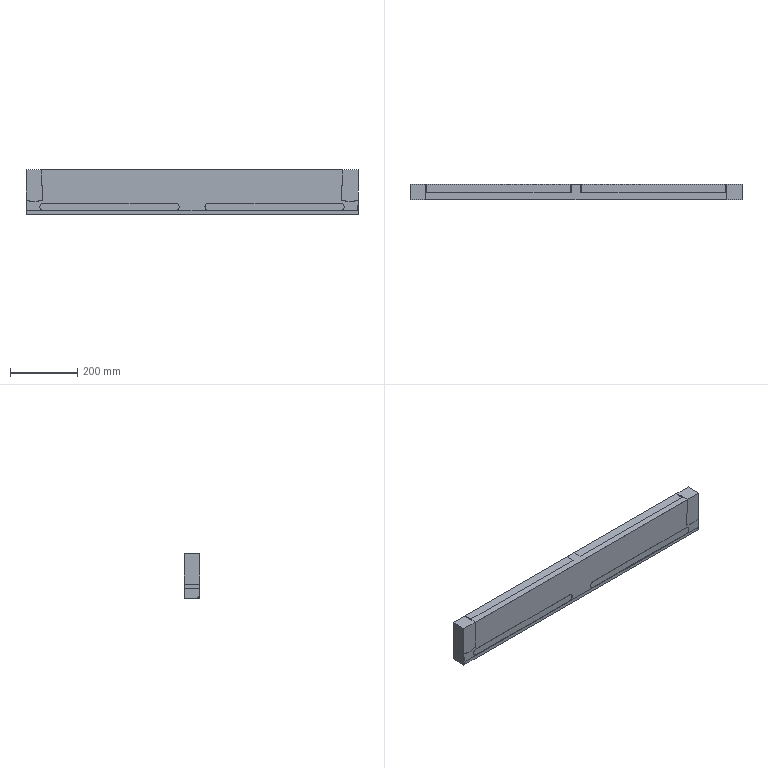NC program | NX | posted with a generic post | part box 987 x 45 x 132.5 mm
Whole program:
N10 G17 G21 G94 G90
(ZLEVEL_PROFILE_2 , TOOL : D12)
N12 T20 M6
N14 G54
N16 G17 G0 G90 X-178.716 Y48.65 B0. C0. S7500 M3
N18 G43 Z30. H20
N20 Z1.5
N22 G94 G1 X-245.5 Z-2. F1001.
N24 X-441. F3000.
N26 G3 X-445.4 Y44.25 R4.4
N28 X-441. Y39.85 R4.4
N30 G1 X-50.
N32 G3 X-45.6 Y44.25 R4.4
N34 X-50. Y48.65 R4.4
N36 G1 X-245.5
N38 X-360.08 Z-4.
N40 X-441.
N42 G3 X-445.4 Y44.25 R4.4
N44 X-441. Y39.85 R4.4
N46 G1 X-50.
N48 G3 X-45.6 Y44.25 R4.4
N50 X-50. Y48.65 R4.4
N52 G1 X-245.5
N54 X-360.08 Z-6.
N56 X-441.
N58 G3 X-445.4 Y44.25 R4.4
N60 X-441. Y39.85 R4.4
N62 G1 X-50.
N64 G3 X-45.6 Y44.25 R4.4
N66 X-50. Y48.65 R4.4
N68 G1 X-245.5
N70 X-360.08 Z-8.
N72 X-441.
N74 G3 X-445.4 Y44.25 R4.4
N76 X-441. Y39.85 R4.4
N78 G1 X-50.
N80 G3 X-45.6 Y44.25 R4.4
N82 X-50. Y48.65 R4.4
N84 G1 X-245.5
N86 X-360.08 Z-10.
N88 X-441.
N90 G3 X-445.4 Y44.25 R4.4
N92 X-441. Y39.85 R4.4
N94 G1 X-50.
N96 G3 X-45.6 Y44.25 R4.4
N98 X-50. Y48.65 R4.4
N100 G1 X-245.5
N102 X-360.08 Z-12.
N104 X-441.
N106 G3 X-445.4 Y44.25 R4.4
N108 X-441. Y39.85 R4.4
N110 G1 X-50.
N112 G3 X-45.6 Y44.25 R4.4
N114 X-50. Y48.65 R4.4
N116 G1 X-245.5
N118 X-360.08 Z-14.
N120 X-441.
N122 G3 X-445.4 Y44.25 R4.4
N124 X-441. Y39.85 R4.4
N126 G1 X-50.
N128 G3 X-45.6 Y44.25 R4.4
N130 X-50. Y48.65 R4.4
N132 G1 X-245.5
N134 X-360.08 Z-16.
N136 X-441.
N138 G3 X-445.4 Y44.25 R4.4
N140 X-441. Y39.85 R4.4
N142 G1 X-50.
N144 G3 X-45.6 Y44.25 R4.4
N146 X-50. Y48.65 R4.4
N148 G1 X-245.5
N150 X-360.08 Z-18.
N152 X-441.
N154 G3 X-445.4 Y44.25 R4.4
N156 X-441. Y39.85 R4.4
N158 G1 X-50.
N160 G3 X-45.6 Y44.25 R4.4
N162 X-50. Y48.65 R4.4
N164 G1 X-245.5
N166 X-360.08 Z-20.
N168 X-441.
N170 G3 X-445.4 Y44.25 R4.4
N172 X-441. Y39.85 R4.4
N174 G1 X-50.
N176 G3 X-45.6 Y44.25 R4.4
N178 X-50. Y48.65 R4.4
N180 G1 X-245.5
N182 X-360.08 Z-22.
N184 X-441.
N186 G3 X-445.4 Y44.25 R4.4
N188 X-441. Y39.85 R4.4
N190 G1 X-50.
N192 G3 X-45.6 Y44.25 R4.4
N194 X-50. Y48.65 R4.4
N196 G1 X-360.08
N198 G3 X-361.119 Y48.05 R1.2
N200 G1 X-361.466 Y47.45
N202 Z-20.8
N204 G0 Z30.
N206 X312.284 Y48.65
N208 Z1.5
N210 G1 X245.5 Z-2. F1001.
N212 X50. F3000.
N214 G3 X45.6 Y44.25 R4.4
N216 X50. Y39.85 R4.4
N218 G1 X441.
N220 G3 X445.4 Y44.25 R4.4
N222 X441. Y48.65 R4.4
N224 G1 X245.5
N226 X130.92 Z-4.
N228 X50.
N230 G3 X45.6 Y44.25 R4.4
N232 X50. Y39.85 R4.4
N234 G1 X441.
N236 G3 X445.4 Y44.25 R4.4
N238 X441. Y48.65 R4.4
N240 G1 X245.5
N242 X130.92 Z-6.
N244 X50.
N246 G3 X45.6 Y44.25 R4.4
N248 X50. Y39.85 R4.4
N250 G1 X441.
N252 G3 X445.4 Y44.25 R4.4
N254 X441. Y48.65 R4.4
N256 G1 X245.5
N258 X130.92 Z-8.
N260 X50.
N262 G3 X45.6 Y44.25 R4.4
N264 X50. Y39.85 R4.4
N266 G1 X441.
N268 G3 X445.4 Y44.25 R4.4
N270 X441. Y48.65 R4.4
N272 G1 X245.5
N274 X130.92 Z-10.
N276 X50.
N278 G3 X45.6 Y44.25 R4.4
N280 X50. Y39.85 R4.4
N282 G1 X441.
N284 G3 X445.4 Y44.25 R4.4
N286 X441. Y48.65 R4.4
N288 G1 X245.5
N290 X130.92 Z-12.
N292 X50.
N294 G3 X45.6 Y44.25 R4.4
N296 X50. Y39.85 R4.4
N298 G1 X441.
N300 G3 X445.4 Y44.25 R4.4
N302 X441. Y48.65 R4.4
N304 G1 X245.5
N306 X130.92 Z-14.
N308 X50.
N310 G3 X45.6 Y44.25 R4.4
N312 X50. Y39.85 R4.4
N314 G1 X441.
N316 G3 X445.4 Y44.25 R4.4
N318 X441. Y48.65 R4.4
N320 G1 X245.5
N322 X130.92 Z-16.
N324 X50.
N326 G3 X45.6 Y44.25 R4.4
N328 X50. Y39.85 R4.4
N330 G1 X441.
N332 G3 X445.4 Y44.25 R4.4
N334 X441. Y48.65 R4.4
N336 G1 X245.5
N338 X130.92 Z-18.
N340 X50.
N342 G3 X45.6 Y44.25 R4.4
N344 X50. Y39.85 R4.4
N346 G1 X441.
N348 G3 X445.4 Y44.25 R4.4
N350 X441. Y48.65 R4.4
N352 G1 X245.5
N354 X130.92 Z-20.
N356 X50.
N358 G3 X45.6 Y44.25 R4.4
N360 X50. Y39.85 R4.4
N362 G1 X441.
N364 G3 X445.4 Y44.25 R4.4
N366 X441. Y48.65 R4.4
N368 G1 X245.5
N370 X130.92 Z-22.
N372 X50.
N374 G3 X45.6 Y44.25 R4.4
N376 X50. Y39.85 R4.4
N378 G1 X441.
N380 G3 X445.4 Y44.25 R4.4
N382 X441. Y48.65 R4.4
N384 G1 X130.92
N386 G3 X129.881 Y48.05 R1.2
N388 G1 X129.534 Y47.45
N390 Z-20.8
N392 G0 Z30.
(11 , TOOL : D12)
N394 X-49.459 Y46.279 S6500
N396 Z-21.
N398 G1 Z-22. F1000.
N400 X-48.961 Y48.15
N402 G3 X-50. Y48.75 R1.2
N404 G1 X-441.
N406 G3 X-445.5 Y44.25 R4.5
N408 X-441. Y39.75 R4.5
N410 G1 X-50.
N412 G3 X-45.5 Y44.25 R4.5
N414 X-50. Y48.75 R4.5
N416 X-51.039 Y48.15 R1.2
N418 G1 X-52.078 Y46.35
N420 Z-21.
N422 G0 Z30.
N424 X441.541 Y46.279
N426 Z-21.
N428 G1 Z-22.
N430 X442.039 Y48.15
N432 G3 X441. Y48.75 R1.2
N434 G1 X50.
N436 G3 X45.5 Y44.25 R4.5
N438 X50. Y39.75 R4.5
N440 G1 X441.
N442 G3 X445.5 Y44.25 R4.5
N444 X441. Y48.75 R4.5
N446 X439.961 Y48.15 R1.2
N448 G1 X438.922 Y46.35
N450 Z-21.
N452 G0 Z30.
N454 M5
(ZLEVEL_PROFILE_1_COPY_1_COPY_COPY_1_COPY_1_COPY_1 , TOOL : D10A45)
N456 T07 M6
N458 G54
N460 G17 G0 G90 X-48.131 Y51.513 B0. C0. S7500 M3
N462 G43 Z30. H7
N464 Z-1.
N466 G94 G1 Z-2. F1000.
N468 X-49.134 Y53.25
N470 G3 X-50. Y53.75 R1.
N472 G1 X-441.
N474 G3 X-450.5 Y44.25 R9.5
N476 X-441. Y34.75 R9.5
N478 G1 X-50.
N480 G3 X-40.5 Y44.25 R9.5
N482 X-50. Y53.75 R9.5
N484 X-50.866 Y53.25 R1.
N486 G1 X-51.732 Y51.75
N488 Z-1.
N490 G0 Z30.
N492 X442.869 Y51.513
N494 Z-1.
N496 G1 Z-2.
N498 X441.866 Y53.25
N500 G3 X441. Y53.75 R1.
N502 G1 X50.
N504 G3 X40.5 Y44.25 R9.5
N506 X50. Y34.75 R9.5
N508 G1 X441.
N510 G3 X450.5 Y44.25 R9.5
N512 X441. Y53.75 R9.5
N514 X440.134 Y53.25 R1.
N516 G1 X439.268 Y51.75
N518 Z-1.
N520 G0 Z30.
(ZLEVEL_PROFILE_1_COPY_1_COPY_COPY_1_COPY_COPY , TOOL : D10A45)
N522 X-449.183 Y-76.003 S7000
N524 Z-0.5
N526 G1 Z-1.5
N528 X-448.063 Y-75.165
N530 G3 X-447.67 Y-74.245 R1.
N532 G1 X-447.693 Y-74.053
N534 Y-18.899
N536 G2 X-446.401 Y-17.607 R1.296
N538 G1 X-444.693
N540 Y24.957
N542 X-457.401
N544 G2 X-458.693 Y26.248 R1.291
N546 G1 Y28.057
N548 X-481.307
N550 Y26.248
N552 G2 X-482.599 Y24.957 R1.291
N554 G1 X-493.001
N556 G2 X-493.914 Y25.335 R1.291
N558 G1 X-494.415 Y25.836
N560 G2 X-494.793 Y26.749 R1.291
N562 G1 Y36.314
N564 X-492.788 Y56.365
N566 X-491.304 Y71.203
N568 G3 X-491.715 Y72.115 R1.
N570 G1 X-492.812 Y72.903
N572 Z-0.5
N574 G0 Z30.
N576 X492.812 Y72.904
N578 Z-0.5
N580 G1 Z-1.5
N582 X491.715 Y72.115
N584 G3 X491.304 Y71.203 R1.
N586 G1 X492.788 Y56.365
N588 X494.793 Y36.314
N590 Y26.749
N592 G2 X494.415 Y25.836 R1.291
N594 G1 X493.914 Y25.335
N596 G2 X493.001 Y24.957 R1.291
N598 G1 X482.599
N600 G2 X481.307 Y26.248 R1.291
N602 G1 Y28.057
N604 X458.693
N606 Y26.248
N608 G2 X457.401 Y24.957 R1.291
N610 G1 X444.693
N612 Y-17.607
N614 X446.401
N616 G2 X447.693 Y-18.899 R1.296
N618 G1 Y-74.053
N620 X447.687 Y-74.104
N622 G3 X448.08 Y-75.024 R1.
N624 G1 X449.247 Y-75.898
N626 Z-0.5
N628 G0 Z30.
N630 M5
(PLANAR_PROFILE_COPY_COPY_COPY , TOOL : D30INNERRCUTTER)
N632 T09 M6
N634 G54
N636 G17 G0 G90 X-497.5 Y77.25 B0. C0. S7500 M3
N638 G43 Z30. H9
N640 Z-7.
N642 G94 G1 Z-10. F1250.
N644 G3 X-491.5 Y74.25 R7.5
N646 G1 X491.5
N648 G3 X497.5 Y77.25 R7.5
N650 G1 Z-7.
N652 G0 Z30.
(PLANAR_PROFILE_COPY_COPY_COPY_COPY , TOOL : D30INNERRCUTTER)
N654 X-497.5 Y76.25
N656 Z-7.
N658 G1 Z-10.
N660 G3 X-491.5 Y73.25 R7.5
N662 G1 X491.5
N664 G3 X497.5 Y76.25 R7.5
N666 G1 Z-7.
N668 G0 Z30.
(PLANAR_PROFILE_COPY_COPY_COPY_COPY_COPY , TOOL : D30INNERRCUTTER)
N670 X-497.5 Y75.25
N672 Z-7.
N674 G1 Z-10.
N676 G3 X-491.5 Y72.25 R7.5
N678 G1 X491.5
N680 G3 X497.5 Y75.25 R7.5
N682 G1 Z-7.
N684 G0 Z30.
(PLANAR_PROFILE_COPY_COPY_COPY_COPY_COPY_COPY , TOOL : D30INNERRCUTTER)
N686 X-497.5 Y74.25
N688 Z-7.
N690 G1 Z-10.
N692 G3 X-491.5 Y71.25 R7.5
N694 G1 X491.5
N696 G3 X497.5 Y74.25 R7.5
N698 G1 Z-7.
N700 G0 Z30.
N702 M5
N704 M2